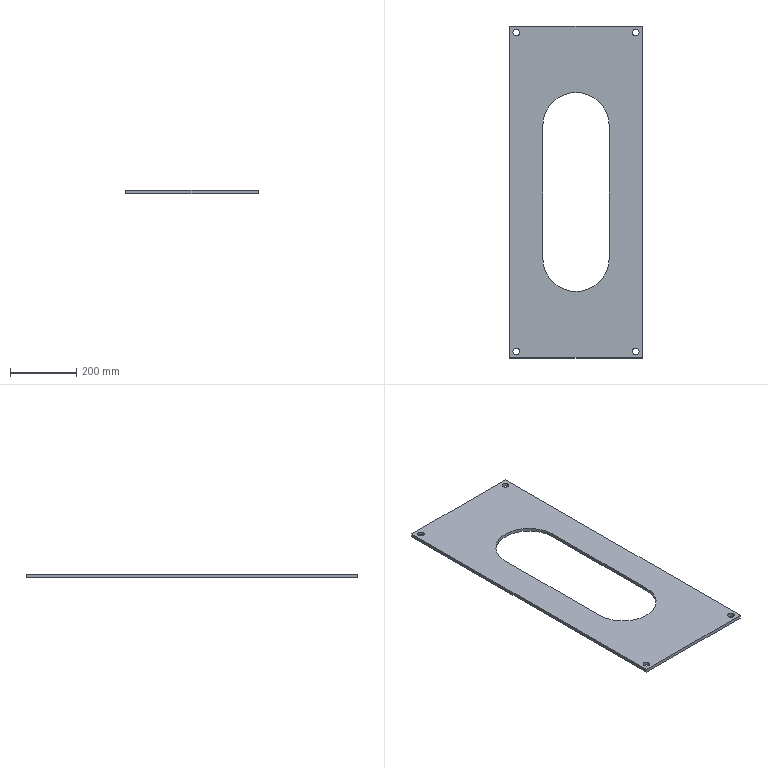Part | SolidWorks | features ICE 2, Extrusion 1 | 1 solid | 18 faces | box 400 x 1000 x 10 mm | volume 2873274 mm3 | cylinder 10 | plane 8 | commonest cylinder face diameters 20 x8 200 x2
STEP:
#1=CARTESIAN_POINT('',(190.,-480.,10.));
#2=VERTEX_POINT('',#1);
#3=CARTESIAN_POINT('',(170.,-480.,10.));
#4=VERTEX_POINT('',#3);
#5=CARTESIAN_POINT('',(180.,-480.,10.));
#6=DIRECTION('',(0.,0.,-1.));
#7=DIRECTION('',(-1.,0.,0.));
#8=AXIS2_PLACEMENT_3D('',#5,#6,#7);
#9=CIRCLE('',#8,10.);
#10=EDGE_CURVE('',#2,#4,#9,.T.);
#11=ORIENTED_EDGE('',*,*,#10,.F.);
#12=CARTESIAN_POINT('',(190.,-480.,0.));
#13=VERTEX_POINT('',#12);
#14=CARTESIAN_POINT('',(190.,-480.,42.));
#15=DIRECTION('',(0.,0.,-1.));
#16=VECTOR('',#15,1000.);
#17=LINE('',#14,#16);
#18=EDGE_CURVE('',#2,#13,#17,.T.);
#19=ORIENTED_EDGE('',*,*,#18,.T.);
#20=CARTESIAN_POINT('',(170.,-480.,0.));
#21=VERTEX_POINT('',#20);
#22=CARTESIAN_POINT('',(180.,-480.,0.));
#23=DIRECTION('',(0.,0.,-1.));
#24=DIRECTION('',(1.,0.,0.));
#25=AXIS2_PLACEMENT_3D('',#22,#23,#24);
#26=CIRCLE('',#25,10.);
#27=EDGE_CURVE('',#13,#21,#26,.T.);
#28=ORIENTED_EDGE('',*,*,#27,.T.);
#29=CARTESIAN_POINT('',(170.,-480.,42.));
#30=DIRECTION('',(0.,0.,-1.));
#31=VECTOR('',#30,1000.);
#32=LINE('',#29,#31);
#33=EDGE_CURVE('',#4,#21,#32,.T.);
#34=ORIENTED_EDGE('',*,*,#33,.F.);
#35=EDGE_LOOP('',(#11,#19,#28,#34));
#36=FACE_OUTER_BOUND('',#35,.T.);
#37=CARTESIAN_POINT('',(180.,-480.,42.));
#38=DIRECTION('',(0.,0.,-1.));
#39=DIRECTION('',(-1.,0.,0.));
#40=AXIS2_PLACEMENT_3D('',#37,#38,#39);
#41=CYLINDRICAL_SURFACE('',#40,10.);
#42=ADVANCED_FACE('',(#36),#41,.F.);
#43=CARTESIAN_POINT('',(-170.,-480.,10.));
#44=VERTEX_POINT('',#43);
#45=CARTESIAN_POINT('',(-190.,-480.,10.));
#46=VERTEX_POINT('',#45);
#47=CARTESIAN_POINT('',(-180.,-480.,10.));
#48=DIRECTION('',(0.,0.,-1.));
#49=DIRECTION('',(-1.,0.,0.));
#50=AXIS2_PLACEMENT_3D('',#47,#48,#49);
#51=CIRCLE('',#50,10.);
#52=EDGE_CURVE('',#44,#46,#51,.T.);
#53=ORIENTED_EDGE('',*,*,#52,.F.);
#54=CARTESIAN_POINT('',(-170.,-480.,0.));
#55=VERTEX_POINT('',#54);
#56=CARTESIAN_POINT('',(-170.,-480.,42.));
#57=DIRECTION('',(0.,0.,-1.));
#58=VECTOR('',#57,1000.);
#59=LINE('',#56,#58);
#60=EDGE_CURVE('',#44,#55,#59,.T.);
#61=ORIENTED_EDGE('',*,*,#60,.T.);
#62=CARTESIAN_POINT('',(-190.,-480.,0.));
#63=VERTEX_POINT('',#62);
#64=CARTESIAN_POINT('',(-180.,-480.,0.));
#65=DIRECTION('',(0.,0.,-1.));
#66=DIRECTION('',(-1.,0.,0.));
#67=AXIS2_PLACEMENT_3D('',#64,#65,#66);
#68=CIRCLE('',#67,10.);
#69=EDGE_CURVE('',#55,#63,#68,.T.);
#70=ORIENTED_EDGE('',*,*,#69,.T.);
#71=CARTESIAN_POINT('',(-190.,-480.,42.));
#72=DIRECTION('',(0.,0.,-1.));
#73=VECTOR('',#72,1000.);
#74=LINE('',#71,#73);
#75=EDGE_CURVE('',#46,#63,#74,.T.);
#76=ORIENTED_EDGE('',*,*,#75,.F.);
#77=EDGE_LOOP('',(#53,#61,#70,#76));
#78=FACE_OUTER_BOUND('',#77,.T.);
#79=CARTESIAN_POINT('',(-180.,-480.,42.));
#80=DIRECTION('',(0.,0.,-1.));
#81=DIRECTION('',(-1.,0.,0.));
#82=AXIS2_PLACEMENT_3D('',#79,#80,#81);
#83=CYLINDRICAL_SURFACE('',#82,10.);
#84=ADVANCED_FACE('',(#78),#83,.F.);
#85=CARTESIAN_POINT('',(-170.,480.,10.));
#86=VERTEX_POINT('',#85);
#87=CARTESIAN_POINT('',(-190.,480.,10.));
#88=VERTEX_POINT('',#87);
#89=CARTESIAN_POINT('',(-180.,480.,10.));
#90=DIRECTION('',(0.,0.,-1.));
#91=DIRECTION('',(-1.,0.,0.));
#92=AXIS2_PLACEMENT_3D('',#89,#90,#91);
#93=CIRCLE('',#92,10.);
#94=EDGE_CURVE('',#86,#88,#93,.T.);
#95=ORIENTED_EDGE('',*,*,#94,.F.);
#96=CARTESIAN_POINT('',(-170.,480.,0.));
#97=VERTEX_POINT('',#96);
#98=CARTESIAN_POINT('',(-170.,480.,42.));
#99=DIRECTION('',(0.,0.,-1.));
#100=VECTOR('',#99,1000.);
#101=LINE('',#98,#100);
#102=EDGE_CURVE('',#86,#97,#101,.T.);
#103=ORIENTED_EDGE('',*,*,#102,.T.);
#104=CARTESIAN_POINT('',(-190.,480.,0.));
#105=VERTEX_POINT('',#104);
#106=CARTESIAN_POINT('',(-180.,480.,0.));
#107=DIRECTION('',(0.,0.,-1.));
#108=DIRECTION('',(1.,0.,0.));
#109=AXIS2_PLACEMENT_3D('',#106,#107,#108);
#110=CIRCLE('',#109,10.);
#111=EDGE_CURVE('',#97,#105,#110,.T.);
#112=ORIENTED_EDGE('',*,*,#111,.T.);
#113=CARTESIAN_POINT('',(-190.,480.,42.));
#114=DIRECTION('',(0.,0.,-1.));
#115=VECTOR('',#114,1000.);
#116=LINE('',#113,#115);
#117=EDGE_CURVE('',#88,#105,#116,.T.);
#118=ORIENTED_EDGE('',*,*,#117,.F.);
#119=EDGE_LOOP('',(#95,#103,#112,#118));
#120=FACE_OUTER_BOUND('',#119,.T.);
#121=CARTESIAN_POINT('',(-180.,480.,42.));
#122=DIRECTION('',(0.,0.,-1.));
#123=DIRECTION('',(-1.,0.,0.));
#124=AXIS2_PLACEMENT_3D('',#121,#122,#123);
#125=CYLINDRICAL_SURFACE('',#124,10.);
#126=ADVANCED_FACE('',(#120),#125,.F.);
#127=CARTESIAN_POINT('',(190.,480.,10.));
#128=VERTEX_POINT('',#127);
#129=CARTESIAN_POINT('',(170.,480.,10.));
#130=VERTEX_POINT('',#129);
#131=CARTESIAN_POINT('',(180.,480.,10.));
#132=DIRECTION('',(0.,0.,-1.));
#133=DIRECTION('',(-1.,0.,0.));
#134=AXIS2_PLACEMENT_3D('',#131,#132,#133);
#135=CIRCLE('',#134,10.);
#136=EDGE_CURVE('',#128,#130,#135,.T.);
#137=ORIENTED_EDGE('',*,*,#136,.F.);
#138=CARTESIAN_POINT('',(190.,480.,0.));
#139=VERTEX_POINT('',#138);
#140=CARTESIAN_POINT('',(190.,480.,42.));
#141=DIRECTION('',(0.,0.,-1.));
#142=VECTOR('',#141,1000.);
#143=LINE('',#140,#142);
#144=EDGE_CURVE('',#128,#139,#143,.T.);
#145=ORIENTED_EDGE('',*,*,#144,.T.);
#146=CARTESIAN_POINT('',(170.,480.,0.));
#147=VERTEX_POINT('',#146);
#148=CARTESIAN_POINT('',(180.,480.,0.));
#149=DIRECTION('',(0.,0.,-1.));
#150=DIRECTION('',(-1.,0.,0.));
#151=AXIS2_PLACEMENT_3D('',#148,#149,#150);
#152=CIRCLE('',#151,10.);
#153=EDGE_CURVE('',#139,#147,#152,.T.);
#154=ORIENTED_EDGE('',*,*,#153,.T.);
#155=CARTESIAN_POINT('',(170.,480.,42.));
#156=DIRECTION('',(0.,0.,-1.));
#157=VECTOR('',#156,1000.);
#158=LINE('',#155,#157);
#159=EDGE_CURVE('',#130,#147,#158,.T.);
#160=ORIENTED_EDGE('',*,*,#159,.F.);
#161=EDGE_LOOP('',(#137,#145,#154,#160));
#162=FACE_OUTER_BOUND('',#161,.T.);
#163=CARTESIAN_POINT('',(180.,480.,42.));
#164=DIRECTION('',(0.,0.,-1.));
#165=DIRECTION('',(-1.,0.,0.));
#166=AXIS2_PLACEMENT_3D('',#163,#164,#165);
#167=CYLINDRICAL_SURFACE('',#166,10.);
#168=ADVANCED_FACE('',(#162),#167,.F.);
#169=CARTESIAN_POINT('',(200.,-500.,0.));
#170=VERTEX_POINT('',#169);
#171=CARTESIAN_POINT('',(200.,500.,0.));
#172=VERTEX_POINT('',#171);
#173=CARTESIAN_POINT('',(200.,-500.,0.));
#174=DIRECTION('',(0.,1.,0.));
#175=VECTOR('',#174,1000.);
#176=LINE('',#173,#175);
#177=EDGE_CURVE('',#170,#172,#176,.T.);
#178=ORIENTED_EDGE('',*,*,#177,.T.);
#179=CARTESIAN_POINT('',(200.,500.,10.));
#180=VERTEX_POINT('',#179);
#181=CARTESIAN_POINT('',(200.,500.,10.));
#182=DIRECTION('',(0.,0.,-1.));
#183=VECTOR('',#182,1000.);
#184=LINE('',#181,#183);
#185=EDGE_CURVE('',#180,#172,#184,.T.);
#186=ORIENTED_EDGE('',*,*,#185,.F.);
#187=CARTESIAN_POINT('',(200.,-500.,10.));
#188=VERTEX_POINT('',#187);
#189=CARTESIAN_POINT('',(200.,-500.,10.));
#190=DIRECTION('',(0.,1.,0.));
#191=VECTOR('',#190,1000.);
#192=LINE('',#189,#191);
#193=EDGE_CURVE('',#188,#180,#192,.T.);
#194=ORIENTED_EDGE('',*,*,#193,.F.);
#195=CARTESIAN_POINT('',(200.,-500.,10.));
#196=DIRECTION('',(0.,0.,-1.));
#197=VECTOR('',#196,1000.);
#198=LINE('',#195,#197);
#199=EDGE_CURVE('',#188,#170,#198,.T.);
#200=ORIENTED_EDGE('',*,*,#199,.T.);
#201=EDGE_LOOP('',(#178,#186,#194,#200));
#202=FACE_OUTER_BOUND('',#201,.T.);
#203=CARTESIAN_POINT('',(200.,-500.,10.));
#204=DIRECTION('',(-1.,0.,0.));
#205=DIRECTION('',(0.,0.,1.));
#206=AXIS2_PLACEMENT_3D('',#203,#204,#205);
#207=PLANE('',#206);
#208=ADVANCED_FACE('',(#202),#207,.F.);
#209=CARTESIAN_POINT('',(-200.,500.,0.));
#210=VERTEX_POINT('',#209);
#211=CARTESIAN_POINT('',(-200.,500.,0.));
#212=DIRECTION('',(-1.,0.,0.));
#213=VECTOR('',#212,1000.);
#214=LINE('',#211,#213);
#215=EDGE_CURVE('',#172,#210,#214,.T.);
#216=ORIENTED_EDGE('',*,*,#215,.T.);
#217=CARTESIAN_POINT('',(-200.,500.,10.));
#218=VERTEX_POINT('',#217);
#219=CARTESIAN_POINT('',(-200.,500.,10.));
#220=DIRECTION('',(0.,0.,-1.));
#221=VECTOR('',#220,1000.);
#222=LINE('',#219,#221);
#223=EDGE_CURVE('',#218,#210,#222,.T.);
#224=ORIENTED_EDGE('',*,*,#223,.F.);
#225=CARTESIAN_POINT('',(-200.,500.,10.));
#226=DIRECTION('',(-1.,0.,0.));
#227=VECTOR('',#226,1000.);
#228=LINE('',#225,#227);
#229=EDGE_CURVE('',#180,#218,#228,.T.);
#230=ORIENTED_EDGE('',*,*,#229,.F.);
#231=ORIENTED_EDGE('',*,*,#185,.T.);
#232=EDGE_LOOP('',(#216,#224,#230,#231));
#233=FACE_OUTER_BOUND('',#232,.T.);
#234=CARTESIAN_POINT('',(-200.,500.,10.));
#235=DIRECTION('',(0.,-1.,0.));
#236=DIRECTION('',(0.,0.,-1.));
#237=AXIS2_PLACEMENT_3D('',#234,#235,#236);
#238=PLANE('',#237);
#239=ADVANCED_FACE('',(#233),#238,.F.);
#240=CARTESIAN_POINT('',(-200.,-500.,0.));
#241=VERTEX_POINT('',#240);
#242=CARTESIAN_POINT('',(-200.,-500.,0.));
#243=DIRECTION('',(0.,-1.,0.));
#244=VECTOR('',#243,1000.);
#245=LINE('',#242,#244);
#246=EDGE_CURVE('',#210,#241,#245,.T.);
#247=ORIENTED_EDGE('',*,*,#246,.T.);
#248=CARTESIAN_POINT('',(-200.,-500.,10.));
#249=VERTEX_POINT('',#248);
#250=CARTESIAN_POINT('',(-200.,-500.,10.));
#251=DIRECTION('',(0.,0.,-1.));
#252=VECTOR('',#251,1000.);
#253=LINE('',#250,#252);
#254=EDGE_CURVE('',#249,#241,#253,.T.);
#255=ORIENTED_EDGE('',*,*,#254,.F.);
#256=CARTESIAN_POINT('',(-200.,-500.,10.));
#257=DIRECTION('',(0.,-1.,0.));
#258=VECTOR('',#257,1000.);
#259=LINE('',#256,#258);
#260=EDGE_CURVE('',#218,#249,#259,.T.);
#261=ORIENTED_EDGE('',*,*,#260,.F.);
#262=ORIENTED_EDGE('',*,*,#223,.T.);
#263=EDGE_LOOP('',(#247,#255,#261,#262));
#264=FACE_OUTER_BOUND('',#263,.T.);
#265=CARTESIAN_POINT('',(-200.,-500.,10.));
#266=DIRECTION('',(1.,0.,0.));
#267=DIRECTION('',(0.,0.,-1.));
#268=AXIS2_PLACEMENT_3D('',#265,#266,#267);
#269=PLANE('',#268);
#270=ADVANCED_FACE('',(#264),#269,.F.);
#271=CARTESIAN_POINT('',(-200.,-500.,0.));
#272=DIRECTION('',(1.,0.,0.));
#273=VECTOR('',#272,1000.);
#274=LINE('',#271,#273);
#275=EDGE_CURVE('',#241,#170,#274,.T.);
#276=ORIENTED_EDGE('',*,*,#275,.T.);
#277=ORIENTED_EDGE('',*,*,#199,.F.);
#278=CARTESIAN_POINT('',(-200.,-500.,10.));
#279=DIRECTION('',(1.,0.,0.));
#280=VECTOR('',#279,1000.);
#281=LINE('',#278,#280);
#282=EDGE_CURVE('',#249,#188,#281,.T.);
#283=ORIENTED_EDGE('',*,*,#282,.F.);
#284=ORIENTED_EDGE('',*,*,#254,.T.);
#285=EDGE_LOOP('',(#276,#277,#283,#284));
#286=FACE_OUTER_BOUND('',#285,.T.);
#287=CARTESIAN_POINT('',(-200.,-500.,10.));
#288=DIRECTION('',(0.,1.,0.));
#289=DIRECTION('',(0.,0.,1.));
#290=AXIS2_PLACEMENT_3D('',#287,#288,#289);
#291=PLANE('',#290);
#292=ADVANCED_FACE('',(#286),#291,.F.);
#293=CARTESIAN_POINT('',(-100.,200.,10.));
#294=VERTEX_POINT('',#293);
#295=CARTESIAN_POINT('',(-100.,-200.,10.));
#296=VERTEX_POINT('',#295);
#297=CARTESIAN_POINT('',(-100.,200.,10.));
#298=DIRECTION('',(0.,-1.,0.));
#299=VECTOR('',#298,1000.);
#300=LINE('',#297,#299);
#301=EDGE_CURVE('',#294,#296,#300,.T.);
#302=ORIENTED_EDGE('',*,*,#301,.F.);
#303=CARTESIAN_POINT('',(100.,200.,10.));
#304=VERTEX_POINT('',#303);
#305=CARTESIAN_POINT('',(0.,200.,10.));
#306=DIRECTION('',(0.,0.,1.));
#307=DIRECTION('',(1.,0.,0.));
#308=AXIS2_PLACEMENT_3D('',#305,#306,#307);
#309=CIRCLE('',#308,100.);
#310=EDGE_CURVE('',#304,#294,#309,.T.);
#311=ORIENTED_EDGE('',*,*,#310,.F.);
#312=CARTESIAN_POINT('',(100.,-200.,10.));
#313=VERTEX_POINT('',#312);
#314=CARTESIAN_POINT('',(100.,200.,10.));
#315=DIRECTION('',(0.,1.,0.));
#316=VECTOR('',#315,1000.);
#317=LINE('',#314,#316);
#318=EDGE_CURVE('',#313,#304,#317,.T.);
#319=ORIENTED_EDGE('',*,*,#318,.F.);
#320=CARTESIAN_POINT('',(0.,-200.,10.));
#321=DIRECTION('',(0.,0.,1.));
#322=DIRECTION('',(1.,0.,0.));
#323=AXIS2_PLACEMENT_3D('',#320,#321,#322);
#324=CIRCLE('',#323,100.);
#325=EDGE_CURVE('',#296,#313,#324,.T.);
#326=ORIENTED_EDGE('',*,*,#325,.F.);
#327=EDGE_LOOP('',(#302,#311,#319,#326));
#328=FACE_BOUND('',#327,.T.);
#329=CARTESIAN_POINT('',(180.,-480.,10.));
#330=DIRECTION('',(0.,0.,-1.));
#331=DIRECTION('',(-1.,0.,0.));
#332=AXIS2_PLACEMENT_3D('',#329,#330,#331);
#333=CIRCLE('',#332,10.);
#334=EDGE_CURVE('',#4,#2,#333,.T.);
#335=ORIENTED_EDGE('',*,*,#334,.T.);
#336=ORIENTED_EDGE('',*,*,#10,.T.);
#337=EDGE_LOOP('',(#335,#336));
#338=FACE_BOUND('',#337,.T.);
#339=CARTESIAN_POINT('',(-180.,-480.,10.));
#340=DIRECTION('',(0.,0.,-1.));
#341=DIRECTION('',(-1.,0.,0.));
#342=AXIS2_PLACEMENT_3D('',#339,#340,#341);
#343=CIRCLE('',#342,10.);
#344=EDGE_CURVE('',#46,#44,#343,.T.);
#345=ORIENTED_EDGE('',*,*,#344,.T.);
#346=ORIENTED_EDGE('',*,*,#52,.T.);
#347=EDGE_LOOP('',(#345,#346));
#348=FACE_BOUND('',#347,.T.);
#349=CARTESIAN_POINT('',(-180.,480.,10.));
#350=DIRECTION('',(0.,0.,-1.));
#351=DIRECTION('',(-1.,0.,0.));
#352=AXIS2_PLACEMENT_3D('',#349,#350,#351);
#353=CIRCLE('',#352,10.);
#354=EDGE_CURVE('',#88,#86,#353,.T.);
#355=ORIENTED_EDGE('',*,*,#354,.T.);
#356=ORIENTED_EDGE('',*,*,#94,.T.);
#357=EDGE_LOOP('',(#355,#356));
#358=FACE_BOUND('',#357,.T.);
#359=CARTESIAN_POINT('',(180.,480.,10.));
#360=DIRECTION('',(0.,0.,-1.));
#361=DIRECTION('',(-1.,0.,0.));
#362=AXIS2_PLACEMENT_3D('',#359,#360,#361);
#363=CIRCLE('',#362,10.);
#364=EDGE_CURVE('',#130,#128,#363,.T.);
#365=ORIENTED_EDGE('',*,*,#364,.T.);
#366=ORIENTED_EDGE('',*,*,#136,.T.);
#367=EDGE_LOOP('',(#365,#366));
#368=FACE_BOUND('',#367,.T.);
#369=ORIENTED_EDGE('',*,*,#193,.T.);
#370=ORIENTED_EDGE('',*,*,#229,.T.);
#371=ORIENTED_EDGE('',*,*,#260,.T.);
#372=ORIENTED_EDGE('',*,*,#282,.T.);
#373=EDGE_LOOP('',(#369,#370,#371,#372));
#374=FACE_OUTER_BOUND('',#373,.T.);
#375=CARTESIAN_POINT('',(0.,0.,10.));
#376=DIRECTION('',(0.,0.,-1.));
#377=DIRECTION('',(-1.,0.,0.));
#378=AXIS2_PLACEMENT_3D('',#375,#376,#377);
#379=PLANE('',#378);
#380=ADVANCED_FACE('',(#328,#338,#348,#358,#368,#374),#379,.F.);
#381=CARTESIAN_POINT('',(-100.,200.,0.));
#382=VERTEX_POINT('',#381);
#383=CARTESIAN_POINT('',(100.,200.,0.));
#384=VERTEX_POINT('',#383);
#385=CARTESIAN_POINT('',(0.,200.,0.));
#386=DIRECTION('',(0.,0.,-1.));
#387=DIRECTION('',(-1.,0.,0.));
#388=AXIS2_PLACEMENT_3D('',#385,#386,#387);
#389=CIRCLE('',#388,100.);
#390=EDGE_CURVE('',#382,#384,#389,.T.);
#391=ORIENTED_EDGE('',*,*,#390,.F.);
#392=CARTESIAN_POINT('',(-100.,-200.,0.));
#393=VERTEX_POINT('',#392);
#394=CARTESIAN_POINT('',(-100.,0.,0.));
#395=DIRECTION('',(0.,1.,0.));
#396=VECTOR('',#395,1000.);
#397=LINE('',#394,#396);
#398=EDGE_CURVE('',#393,#382,#397,.T.);
#399=ORIENTED_EDGE('',*,*,#398,.F.);
#400=CARTESIAN_POINT('',(100.,-200.,0.));
#401=VERTEX_POINT('',#400);
#402=CARTESIAN_POINT('',(0.,-200.,0.));
#403=DIRECTION('',(0.,0.,-1.));
#404=DIRECTION('',(-1.,0.,0.));
#405=AXIS2_PLACEMENT_3D('',#402,#403,#404);
#406=CIRCLE('',#405,100.);
#407=EDGE_CURVE('',#401,#393,#406,.T.);
#408=ORIENTED_EDGE('',*,*,#407,.F.);
#409=CARTESIAN_POINT('',(100.,0.,0.));
#410=DIRECTION('',(0.,-1.,0.));
#411=VECTOR('',#410,1000.);
#412=LINE('',#409,#411);
#413=EDGE_CURVE('',#384,#401,#412,.T.);
#414=ORIENTED_EDGE('',*,*,#413,.F.);
#415=EDGE_LOOP('',(#391,#399,#408,#414));
#416=FACE_BOUND('',#415,.T.);
#417=CARTESIAN_POINT('',(180.,-480.,0.));
#418=DIRECTION('',(0.,0.,-1.));
#419=DIRECTION('',(1.,0.,0.));
#420=AXIS2_PLACEMENT_3D('',#417,#418,#419);
#421=CIRCLE('',#420,10.);
#422=EDGE_CURVE('',#21,#13,#421,.T.);
#423=ORIENTED_EDGE('',*,*,#422,.F.);
#424=ORIENTED_EDGE('',*,*,#27,.F.);
#425=EDGE_LOOP('',(#423,#424));
#426=FACE_BOUND('',#425,.T.);
#427=CARTESIAN_POINT('',(-180.,-480.,0.));
#428=DIRECTION('',(0.,0.,-1.));
#429=DIRECTION('',(-1.,0.,0.));
#430=AXIS2_PLACEMENT_3D('',#427,#428,#429);
#431=CIRCLE('',#430,10.);
#432=EDGE_CURVE('',#63,#55,#431,.T.);
#433=ORIENTED_EDGE('',*,*,#432,.F.);
#434=ORIENTED_EDGE('',*,*,#69,.F.);
#435=EDGE_LOOP('',(#433,#434));
#436=FACE_BOUND('',#435,.T.);
#437=CARTESIAN_POINT('',(-180.,480.,0.));
#438=DIRECTION('',(0.,0.,-1.));
#439=DIRECTION('',(1.,0.,0.));
#440=AXIS2_PLACEMENT_3D('',#437,#438,#439);
#441=CIRCLE('',#440,10.);
#442=EDGE_CURVE('',#105,#97,#441,.T.);
#443=ORIENTED_EDGE('',*,*,#442,.F.);
#444=ORIENTED_EDGE('',*,*,#111,.F.);
#445=EDGE_LOOP('',(#443,#444));
#446=FACE_BOUND('',#445,.T.);
#447=CARTESIAN_POINT('',(180.,480.,0.));
#448=DIRECTION('',(0.,0.,-1.));
#449=DIRECTION('',(-1.,0.,0.));
#450=AXIS2_PLACEMENT_3D('',#447,#448,#449);
#451=CIRCLE('',#450,10.);
#452=EDGE_CURVE('',#147,#139,#451,.T.);
#453=ORIENTED_EDGE('',*,*,#452,.F.);
#454=ORIENTED_EDGE('',*,*,#153,.F.);
#455=EDGE_LOOP('',(#453,#454));
#456=FACE_BOUND('',#455,.T.);
#457=ORIENTED_EDGE('',*,*,#177,.F.);
#458=ORIENTED_EDGE('',*,*,#275,.F.);
#459=ORIENTED_EDGE('',*,*,#246,.F.);
#460=ORIENTED_EDGE('',*,*,#215,.F.);
#461=EDGE_LOOP('',(#457,#458,#459,#460));
#462=FACE_OUTER_BOUND('',#461,.T.);
#463=CARTESIAN_POINT('',(0.,0.,0.));
#464=DIRECTION('',(0.,0.,-1.));
#465=DIRECTION('',(-1.,0.,0.));
#466=AXIS2_PLACEMENT_3D('',#463,#464,#465);
#467=PLANE('',#466);
#468=ADVANCED_FACE('',(#416,#426,#436,#446,#456,#462),#467,.T.);
#469=ORIENTED_EDGE('',*,*,#144,.F.);
#470=ORIENTED_EDGE('',*,*,#364,.F.);
#471=ORIENTED_EDGE('',*,*,#159,.T.);
#472=ORIENTED_EDGE('',*,*,#452,.T.);
#473=EDGE_LOOP('',(#469,#470,#471,#472));
#474=FACE_OUTER_BOUND('',#473,.T.);
#475=CARTESIAN_POINT('',(180.,480.,42.));
#476=DIRECTION('',(0.,0.,-1.));
#477=DIRECTION('',(-1.,0.,0.));
#478=AXIS2_PLACEMENT_3D('',#475,#476,#477);
#479=CYLINDRICAL_SURFACE('',#478,10.);
#480=ADVANCED_FACE('',(#474),#479,.F.);
#481=ORIENTED_EDGE('',*,*,#102,.F.);
#482=ORIENTED_EDGE('',*,*,#354,.F.);
#483=ORIENTED_EDGE('',*,*,#117,.T.);
#484=ORIENTED_EDGE('',*,*,#442,.T.);
#485=EDGE_LOOP('',(#481,#482,#483,#484));
#486=FACE_OUTER_BOUND('',#485,.T.);
#487=CARTESIAN_POINT('',(-180.,480.,42.));
#488=DIRECTION('',(0.,0.,-1.));
#489=DIRECTION('',(-1.,0.,0.));
#490=AXIS2_PLACEMENT_3D('',#487,#488,#489);
#491=CYLINDRICAL_SURFACE('',#490,10.);
#492=ADVANCED_FACE('',(#486),#491,.F.);
#493=ORIENTED_EDGE('',*,*,#60,.F.);
#494=ORIENTED_EDGE('',*,*,#344,.F.);
#495=ORIENTED_EDGE('',*,*,#75,.T.);
#496=ORIENTED_EDGE('',*,*,#432,.T.);
#497=EDGE_LOOP('',(#493,#494,#495,#496));
#498=FACE_OUTER_BOUND('',#497,.T.);
#499=CARTESIAN_POINT('',(-180.,-480.,42.));
#500=DIRECTION('',(0.,0.,-1.));
#501=DIRECTION('',(-1.,0.,0.));
#502=AXIS2_PLACEMENT_3D('',#499,#500,#501);
#503=CYLINDRICAL_SURFACE('',#502,10.);
#504=ADVANCED_FACE('',(#498),#503,.F.);
#505=ORIENTED_EDGE('',*,*,#18,.F.);
#506=ORIENTED_EDGE('',*,*,#334,.F.);
#507=ORIENTED_EDGE('',*,*,#33,.T.);
#508=ORIENTED_EDGE('',*,*,#422,.T.);
#509=EDGE_LOOP('',(#505,#506,#507,#508));
#510=FACE_OUTER_BOUND('',#509,.T.);
#511=CARTESIAN_POINT('',(180.,-480.,42.));
#512=DIRECTION('',(0.,0.,-1.));
#513=DIRECTION('',(-1.,0.,0.));
#514=AXIS2_PLACEMENT_3D('',#511,#512,#513);
#515=CYLINDRICAL_SURFACE('',#514,10.);
#516=ADVANCED_FACE('',(#510),#515,.F.);
#517=ORIENTED_EDGE('',*,*,#390,.T.);
#518=CARTESIAN_POINT('',(100.,200.,-10.));
#519=DIRECTION('',(0.,0.,1.));
#520=VECTOR('',#519,1000.);
#521=LINE('',#518,#520);
#522=EDGE_CURVE('',#384,#304,#521,.T.);
#523=ORIENTED_EDGE('',*,*,#522,.T.);
#524=ORIENTED_EDGE('',*,*,#310,.T.);
#525=CARTESIAN_POINT('',(-100.,200.,-10.));
#526=DIRECTION('',(0.,0.,1.));
#527=VECTOR('',#526,1000.);
#528=LINE('',#525,#527);
#529=EDGE_CURVE('',#382,#294,#528,.T.);
#530=ORIENTED_EDGE('',*,*,#529,.F.);
#531=EDGE_LOOP('',(#517,#523,#524,#530));
#532=FACE_OUTER_BOUND('',#531,.T.);
#533=CARTESIAN_POINT('',(0.,200.,-10.));
#534=DIRECTION('',(0.,0.,1.));
#535=DIRECTION('',(1.,0.,0.));
#536=AXIS2_PLACEMENT_3D('',#533,#534,#535);
#537=CYLINDRICAL_SURFACE('',#536,100.);
#538=ADVANCED_FACE('',(#532),#537,.F.);
#539=ORIENTED_EDGE('',*,*,#413,.T.);
#540=CARTESIAN_POINT('',(100.,-200.,-10.));
#541=DIRECTION('',(0.,0.,1.));
#542=VECTOR('',#541,1000.);
#543=LINE('',#540,#542);
#544=EDGE_CURVE('',#401,#313,#543,.T.);
#545=ORIENTED_EDGE('',*,*,#544,.T.);
#546=ORIENTED_EDGE('',*,*,#318,.T.);
#547=ORIENTED_EDGE('',*,*,#522,.F.);
#548=EDGE_LOOP('',(#539,#545,#546,#547));
#549=FACE_OUTER_BOUND('',#548,.T.);
#550=CARTESIAN_POINT('',(100.,200.,-10.));
#551=DIRECTION('',(1.,0.,0.));
#552=DIRECTION('',(0.,1.,0.));
#553=AXIS2_PLACEMENT_3D('',#550,#551,#552);
#554=PLANE('',#553);
#555=ADVANCED_FACE('',(#549),#554,.F.);
#556=ORIENTED_EDGE('',*,*,#407,.T.);
#557=CARTESIAN_POINT('',(-100.,-200.,-10.));
#558=DIRECTION('',(0.,0.,1.));
#559=VECTOR('',#558,1000.);
#560=LINE('',#557,#559);
#561=EDGE_CURVE('',#393,#296,#560,.T.);
#562=ORIENTED_EDGE('',*,*,#561,.T.);
#563=ORIENTED_EDGE('',*,*,#325,.T.);
#564=ORIENTED_EDGE('',*,*,#544,.F.);
#565=EDGE_LOOP('',(#556,#562,#563,#564));
#566=FACE_OUTER_BOUND('',#565,.T.);
#567=CARTESIAN_POINT('',(0.,-200.,-10.));
#568=DIRECTION('',(0.,0.,1.));
#569=DIRECTION('',(1.,0.,0.));
#570=AXIS2_PLACEMENT_3D('',#567,#568,#569);
#571=CYLINDRICAL_SURFACE('',#570,100.);
#572=ADVANCED_FACE('',(#566),#571,.F.);
#573=ORIENTED_EDGE('',*,*,#398,.T.);
#574=ORIENTED_EDGE('',*,*,#529,.T.);
#575=ORIENTED_EDGE('',*,*,#301,.T.);
#576=ORIENTED_EDGE('',*,*,#561,.F.);
#577=EDGE_LOOP('',(#573,#574,#575,#576));
#578=FACE_OUTER_BOUND('',#577,.T.);
#579=CARTESIAN_POINT('',(-100.,200.,-10.));
#580=DIRECTION('',(-1.,0.,0.));
#581=DIRECTION('',(0.,-1.,0.));
#582=AXIS2_PLACEMENT_3D('',#579,#580,#581);
#583=PLANE('',#582);
#584=ADVANCED_FACE('',(#578),#583,.F.);
#585=CLOSED_SHELL('',(#42,#84,#126,#168,#208,#239,#270,#292,#380,#468,#480,#492,#504,#516,#538,#555,#572,#584));
#586=MANIFOLD_SOLID_BREP('',#585);
#587=CARTESIAN_POINT('',(0.,0.,0.));
#588=DIRECTION('',(0.,0.,1.));
#589=DIRECTION('',(1.,0.,0.));
#590=AXIS2_PLACEMENT_3D('',#587,#588,#589);
#591=(LENGTH_UNIT()NAMED_UNIT(*)SI_UNIT(.MILLI.,.METRE.));
#592=UNCERTAINTY_MEASURE_WITH_UNIT(LENGTH_MEASURE(0.00001),#591,'','');
#593=(NAMED_UNIT(*)PLANE_ANGLE_UNIT()SI_UNIT($,.RADIAN.));
#594=(NAMED_UNIT(*)SI_UNIT($,.STERADIAN.)SOLID_ANGLE_UNIT());
#595=(GEOMETRIC_REPRESENTATION_CONTEXT(3)GLOBAL_UNCERTAINTY_ASSIGNED_CONTEXT((#592))GLOBAL_UNIT_ASSIGNED_CONTEXT((#591,#593,#594))REPRESENTATION_CONTEXT('',''));
#596=ADVANCED_BREP_SHAPE_REPRESENTATION('',(#586,#590),#595);